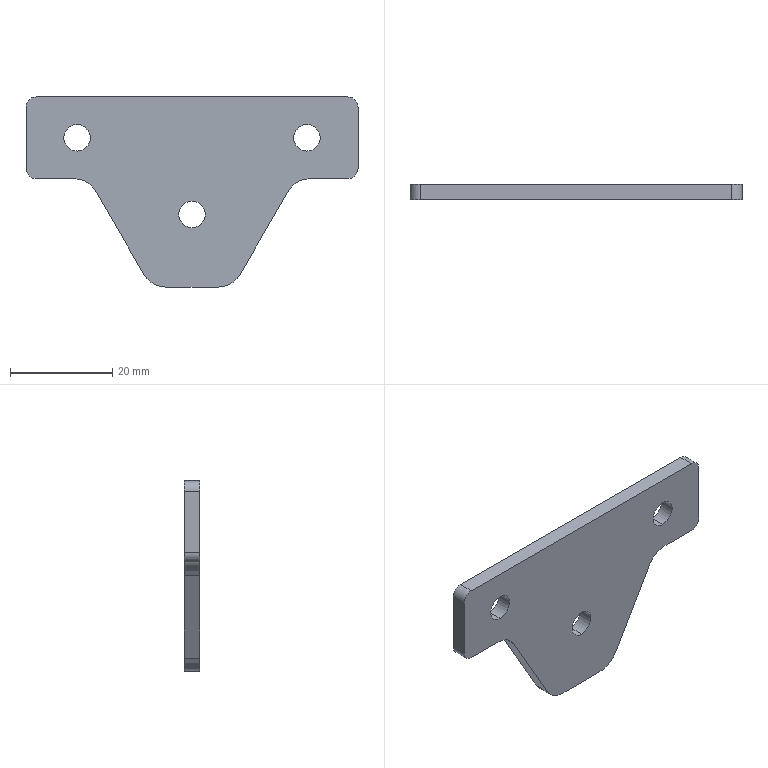Part | SolidWorks | features BaseBody 1 | 1 solid | 24 faces | box 65 x 3 x 37.218 mm | volume 4717 mm3 | cylinder 14 | plane 10 | commonest cylinder face diameters 5.2 x6 4 x4 10 x4
STEP:
#1=CARTESIAN_POINT('',(0.,0.,-17.6));
#2=VERTEX_POINT('',#1);
#3=CARTESIAN_POINT('',(0.,0.,-12.4));
#4=VERTEX_POINT('',#3);
#5=CARTESIAN_POINT('',(0.,0.,-15.));
#6=DIRECTION('',(0.,1.,0.));
#7=DIRECTION('',(0.,0.,1.));
#8=AXIS2_PLACEMENT_3D('',#5,#6,#7);
#9=CIRCLE('',#8,2.6);
#10=EDGE_CURVE('',#2,#4,#9,.T.);
#11=ORIENTED_EDGE('',*,*,#10,.F.);
#12=CARTESIAN_POINT('',(0.,3.,-17.6));
#13=VERTEX_POINT('',#12);
#14=CARTESIAN_POINT('',(0.,0.,-17.6));
#15=DIRECTION('',(0.,1.,0.));
#16=VECTOR('',#15,1000.);
#17=LINE('',#14,#16);
#18=EDGE_CURVE('',#2,#13,#17,.T.);
#19=ORIENTED_EDGE('',*,*,#18,.T.);
#20=CARTESIAN_POINT('',(0.,3.,-12.4));
#21=VERTEX_POINT('',#20);
#22=CARTESIAN_POINT('',(0.,3.,-15.));
#23=DIRECTION('',(0.,-1.,0.));
#24=DIRECTION('',(0.,0.,1.));
#25=AXIS2_PLACEMENT_3D('',#22,#23,#24);
#26=CIRCLE('',#25,2.6);
#27=EDGE_CURVE('',#21,#13,#26,.T.);
#28=ORIENTED_EDGE('',*,*,#27,.F.);
#29=CARTESIAN_POINT('',(0.,0.,-12.4));
#30=DIRECTION('',(0.,1.,0.));
#31=VECTOR('',#30,1000.);
#32=LINE('',#29,#31);
#33=EDGE_CURVE('',#4,#21,#32,.T.);
#34=ORIENTED_EDGE('',*,*,#33,.F.);
#35=EDGE_LOOP('',(#11,#19,#28,#34));
#36=FACE_OUTER_BOUND('',#35,.T.);
#37=CARTESIAN_POINT('',(0.,0.,-15.));
#38=DIRECTION('',(0.,1.,0.));
#39=DIRECTION('',(0.,0.,1.));
#40=AXIS2_PLACEMENT_3D('',#37,#38,#39);
#41=CYLINDRICAL_SURFACE('',#40,2.6);
#42=ADVANCED_FACE('',(#36),#41,.F.);
#43=CARTESIAN_POINT('',(22.5,0.,-2.6));
#44=VERTEX_POINT('',#43);
#45=CARTESIAN_POINT('',(22.5,0.,2.6));
#46=VERTEX_POINT('',#45);
#47=CARTESIAN_POINT('',(22.5,0.,0.));
#48=DIRECTION('',(0.,1.,0.));
#49=DIRECTION('',(0.,0.,1.));
#50=AXIS2_PLACEMENT_3D('',#47,#48,#49);
#51=CIRCLE('',#50,2.6);
#52=EDGE_CURVE('',#44,#46,#51,.T.);
#53=ORIENTED_EDGE('',*,*,#52,.F.);
#54=CARTESIAN_POINT('',(22.5,3.,-2.6));
#55=VERTEX_POINT('',#54);
#56=CARTESIAN_POINT('',(22.5,0.,-2.6));
#57=DIRECTION('',(0.,1.,0.));
#58=VECTOR('',#57,1000.);
#59=LINE('',#56,#58);
#60=EDGE_CURVE('',#44,#55,#59,.T.);
#61=ORIENTED_EDGE('',*,*,#60,.T.);
#62=CARTESIAN_POINT('',(22.5,3.,2.6));
#63=VERTEX_POINT('',#62);
#64=CARTESIAN_POINT('',(22.5,3.,0.));
#65=DIRECTION('',(0.,-1.,0.));
#66=DIRECTION('',(0.,0.,1.));
#67=AXIS2_PLACEMENT_3D('',#64,#65,#66);
#68=CIRCLE('',#67,2.6);
#69=EDGE_CURVE('',#63,#55,#68,.T.);
#70=ORIENTED_EDGE('',*,*,#69,.F.);
#71=CARTESIAN_POINT('',(22.5,0.,2.6));
#72=DIRECTION('',(0.,1.,0.));
#73=VECTOR('',#72,1000.);
#74=LINE('',#71,#73);
#75=EDGE_CURVE('',#46,#63,#74,.T.);
#76=ORIENTED_EDGE('',*,*,#75,.F.);
#77=EDGE_LOOP('',(#53,#61,#70,#76));
#78=FACE_OUTER_BOUND('',#77,.T.);
#79=CARTESIAN_POINT('',(22.5,0.,0.));
#80=DIRECTION('',(0.,1.,0.));
#81=DIRECTION('',(0.,0.,1.));
#82=AXIS2_PLACEMENT_3D('',#79,#80,#81);
#83=CYLINDRICAL_SURFACE('',#82,2.6);
#84=ADVANCED_FACE('',(#78),#83,.F.);
#85=CARTESIAN_POINT('',(-22.5,0.,-2.6));
#86=VERTEX_POINT('',#85);
#87=CARTESIAN_POINT('',(-22.5,0.,2.6));
#88=VERTEX_POINT('',#87);
#89=CARTESIAN_POINT('',(-22.5,0.,0.));
#90=DIRECTION('',(0.,1.,0.));
#91=DIRECTION('',(0.,0.,1.));
#92=AXIS2_PLACEMENT_3D('',#89,#90,#91);
#93=CIRCLE('',#92,2.6);
#94=EDGE_CURVE('',#86,#88,#93,.T.);
#95=ORIENTED_EDGE('',*,*,#94,.F.);
#96=CARTESIAN_POINT('',(-22.5,3.,-2.6));
#97=VERTEX_POINT('',#96);
#98=CARTESIAN_POINT('',(-22.5,0.,-2.6));
#99=DIRECTION('',(0.,1.,0.));
#100=VECTOR('',#99,1000.);
#101=LINE('',#98,#100);
#102=EDGE_CURVE('',#86,#97,#101,.T.);
#103=ORIENTED_EDGE('',*,*,#102,.T.);
#104=CARTESIAN_POINT('',(-22.5,3.,2.6));
#105=VERTEX_POINT('',#104);
#106=CARTESIAN_POINT('',(-22.5,3.,0.));
#107=DIRECTION('',(0.,-1.,0.));
#108=DIRECTION('',(0.,0.,1.));
#109=AXIS2_PLACEMENT_3D('',#106,#107,#108);
#110=CIRCLE('',#109,2.6);
#111=EDGE_CURVE('',#105,#97,#110,.T.);
#112=ORIENTED_EDGE('',*,*,#111,.F.);
#113=CARTESIAN_POINT('',(-22.5,0.,2.6));
#114=DIRECTION('',(0.,1.,0.));
#115=VECTOR('',#114,1000.);
#116=LINE('',#113,#115);
#117=EDGE_CURVE('',#88,#105,#116,.T.);
#118=ORIENTED_EDGE('',*,*,#117,.F.);
#119=EDGE_LOOP('',(#95,#103,#112,#118));
#120=FACE_OUTER_BOUND('',#119,.T.);
#121=CARTESIAN_POINT('',(-22.5,0.,0.));
#122=DIRECTION('',(0.,1.,0.));
#123=DIRECTION('',(0.,0.,1.));
#124=AXIS2_PLACEMENT_3D('',#121,#122,#123);
#125=CYLINDRICAL_SURFACE('',#124,2.6);
#126=ADVANCED_FACE('',(#120),#125,.F.);
#127=ORIENTED_EDGE('',*,*,#27,.T.);
#128=CARTESIAN_POINT('',(0.,3.,-15.));
#129=DIRECTION('',(0.,-1.,0.));
#130=DIRECTION('',(0.,0.,1.));
#131=AXIS2_PLACEMENT_3D('',#128,#129,#130);
#132=CIRCLE('',#131,2.6);
#133=EDGE_CURVE('',#13,#21,#132,.T.);
#134=ORIENTED_EDGE('',*,*,#133,.T.);
#135=EDGE_LOOP('',(#127,#134));
#136=FACE_BOUND('',#135,.T.);
#137=ORIENTED_EDGE('',*,*,#69,.T.);
#138=CARTESIAN_POINT('',(22.5,3.,0.));
#139=DIRECTION('',(0.,-1.,0.));
#140=DIRECTION('',(0.,0.,1.));
#141=AXIS2_PLACEMENT_3D('',#138,#139,#140);
#142=CIRCLE('',#141,2.6);
#143=EDGE_CURVE('',#55,#63,#142,.T.);
#144=ORIENTED_EDGE('',*,*,#143,.T.);
#145=EDGE_LOOP('',(#137,#144));
#146=FACE_BOUND('',#145,.T.);
#147=ORIENTED_EDGE('',*,*,#111,.T.);
#148=CARTESIAN_POINT('',(-22.5,3.,0.));
#149=DIRECTION('',(0.,-1.,0.));
#150=DIRECTION('',(0.,0.,1.));
#151=AXIS2_PLACEMENT_3D('',#148,#149,#150);
#152=CIRCLE('',#151,2.6);
#153=EDGE_CURVE('',#97,#105,#152,.T.);
#154=ORIENTED_EDGE('',*,*,#153,.T.);
#155=EDGE_LOOP('',(#147,#154));
#156=FACE_BOUND('',#155,.T.);
#157=CARTESIAN_POINT('',(30.5,3.,-8.));
#158=VERTEX_POINT('',#157);
#159=CARTESIAN_POINT('',(23.137,3.,-8.));
#160=VERTEX_POINT('',#159);
#161=CARTESIAN_POINT('',(0.,3.,-8.));
#162=DIRECTION('',(-1.,0.,0.));
#163=VECTOR('',#162,1000.);
#164=LINE('',#161,#163);
#165=EDGE_CURVE('',#158,#160,#164,.T.);
#166=ORIENTED_EDGE('',*,*,#165,.T.);
#167=CARTESIAN_POINT('',(18.807,3.,-10.5));
#168=VERTEX_POINT('',#167);
#169=CARTESIAN_POINT('',(23.137,3.,-13.));
#170=DIRECTION('',(0.,-1.,0.));
#171=DIRECTION('',(0.,0.,-1.));
#172=AXIS2_PLACEMENT_3D('',#169,#170,#171);
#173=CIRCLE('',#172,5.);
#174=EDGE_CURVE('',#160,#168,#173,.T.);
#175=ORIENTED_EDGE('',*,*,#174,.T.);
#176=CARTESIAN_POINT('',(9.443,3.,-26.718));
#177=VERTEX_POINT('',#176);
#178=CARTESIAN_POINT('',(18.807,3.,-10.5));
#179=DIRECTION('',(-0.5,0.,-0.866));
#180=VECTOR('',#179,1000.);
#181=LINE('',#178,#180);
#182=EDGE_CURVE('',#168,#177,#181,.T.);
#183=ORIENTED_EDGE('',*,*,#182,.T.);
#184=CARTESIAN_POINT('',(5.113,3.,-29.218));
#185=VERTEX_POINT('',#184);
#186=CARTESIAN_POINT('',(5.113,3.,-24.218));
#187=DIRECTION('',(0.,1.,0.));
#188=DIRECTION('',(0.,0.,-1.));
#189=AXIS2_PLACEMENT_3D('',#186,#187,#188);
#190=CIRCLE('',#189,5.);
#191=EDGE_CURVE('',#177,#185,#190,.T.);
#192=ORIENTED_EDGE('',*,*,#191,.T.);
#193=CARTESIAN_POINT('',(-5.113,3.,-29.218));
#194=VERTEX_POINT('',#193);
#195=CARTESIAN_POINT('',(0.,3.,-29.218));
#196=DIRECTION('',(-1.,0.,0.));
#197=VECTOR('',#196,1000.);
#198=LINE('',#195,#197);
#199=EDGE_CURVE('',#185,#194,#198,.T.);
#200=ORIENTED_EDGE('',*,*,#199,.T.);
#201=CARTESIAN_POINT('',(-9.443,3.,-26.718));
#202=VERTEX_POINT('',#201);
#203=CARTESIAN_POINT('',(-5.113,3.,-24.218));
#204=DIRECTION('',(0.,1.,0.));
#205=DIRECTION('',(0.,0.,1.));
#206=AXIS2_PLACEMENT_3D('',#203,#204,#205);
#207=CIRCLE('',#206,5.);
#208=EDGE_CURVE('',#194,#202,#207,.T.);
#209=ORIENTED_EDGE('',*,*,#208,.T.);
#210=CARTESIAN_POINT('',(-18.807,3.,-10.5));
#211=VERTEX_POINT('',#210);
#212=CARTESIAN_POINT('',(-9.443,3.,-26.718));
#213=DIRECTION('',(-0.5,0.,0.866));
#214=VECTOR('',#213,1000.);
#215=LINE('',#212,#214);
#216=EDGE_CURVE('',#202,#211,#215,.T.);
#217=ORIENTED_EDGE('',*,*,#216,.T.);
#218=CARTESIAN_POINT('',(-23.137,3.,-8.));
#219=VERTEX_POINT('',#218);
#220=CARTESIAN_POINT('',(-23.137,3.,-13.));
#221=DIRECTION('',(0.,-1.,0.));
#222=DIRECTION('',(0.,0.,1.));
#223=AXIS2_PLACEMENT_3D('',#220,#221,#222);
#224=CIRCLE('',#223,5.);
#225=EDGE_CURVE('',#211,#219,#224,.T.);
#226=ORIENTED_EDGE('',*,*,#225,.T.);
#227=CARTESIAN_POINT('',(-30.5,3.,-8.));
#228=VERTEX_POINT('',#227);
#229=CARTESIAN_POINT('',(0.,3.,-8.));
#230=DIRECTION('',(-1.,0.,0.));
#231=VECTOR('',#230,1000.);
#232=LINE('',#229,#231);
#233=EDGE_CURVE('',#219,#228,#232,.T.);
#234=ORIENTED_EDGE('',*,*,#233,.T.);
#235=CARTESIAN_POINT('',(-32.5,3.,-6.));
#236=VERTEX_POINT('',#235);
#237=CARTESIAN_POINT('',(-30.5,3.,-6.));
#238=DIRECTION('',(0.,1.,0.));
#239=DIRECTION('',(0.,0.,-1.));
#240=AXIS2_PLACEMENT_3D('',#237,#238,#239);
#241=CIRCLE('',#240,2.);
#242=EDGE_CURVE('',#228,#236,#241,.T.);
#243=ORIENTED_EDGE('',*,*,#242,.T.);
#244=CARTESIAN_POINT('',(-32.5,3.,6.));
#245=VERTEX_POINT('',#244);
#246=CARTESIAN_POINT('',(-32.5,3.,0.));
#247=DIRECTION('',(0.,0.,1.));
#248=VECTOR('',#247,1000.);
#249=LINE('',#246,#248);
#250=EDGE_CURVE('',#236,#245,#249,.T.);
#251=ORIENTED_EDGE('',*,*,#250,.T.);
#252=CARTESIAN_POINT('',(-30.5,3.,8.));
#253=VERTEX_POINT('',#252);
#254=CARTESIAN_POINT('',(-30.5,3.,6.));
#255=DIRECTION('',(0.,1.,0.));
#256=DIRECTION('',(0.,0.,1.));
#257=AXIS2_PLACEMENT_3D('',#254,#255,#256);
#258=CIRCLE('',#257,2.);
#259=EDGE_CURVE('',#245,#253,#258,.T.);
#260=ORIENTED_EDGE('',*,*,#259,.T.);
#261=CARTESIAN_POINT('',(30.5,3.,8.));
#262=VERTEX_POINT('',#261);
#263=CARTESIAN_POINT('',(0.,3.,8.));
#264=DIRECTION('',(1.,0.,0.));
#265=VECTOR('',#264,1000.);
#266=LINE('',#263,#265);
#267=EDGE_CURVE('',#253,#262,#266,.T.);
#268=ORIENTED_EDGE('',*,*,#267,.T.);
#269=CARTESIAN_POINT('',(32.5,3.,6.));
#270=VERTEX_POINT('',#269);
#271=CARTESIAN_POINT('',(30.5,3.,6.));
#272=DIRECTION('',(0.,1.,0.));
#273=DIRECTION('',(0.,0.,-1.));
#274=AXIS2_PLACEMENT_3D('',#271,#272,#273);
#275=CIRCLE('',#274,2.);
#276=EDGE_CURVE('',#262,#270,#275,.T.);
#277=ORIENTED_EDGE('',*,*,#276,.T.);
#278=CARTESIAN_POINT('',(32.5,3.,-6.));
#279=VERTEX_POINT('',#278);
#280=CARTESIAN_POINT('',(32.5,3.,0.));
#281=DIRECTION('',(0.,0.,-1.));
#282=VECTOR('',#281,1000.);
#283=LINE('',#280,#282);
#284=EDGE_CURVE('',#270,#279,#283,.T.);
#285=ORIENTED_EDGE('',*,*,#284,.T.);
#286=CARTESIAN_POINT('',(30.5,3.,-6.));
#287=DIRECTION('',(0.,1.,0.));
#288=DIRECTION('',(0.,0.,1.));
#289=AXIS2_PLACEMENT_3D('',#286,#287,#288);
#290=CIRCLE('',#289,2.);
#291=EDGE_CURVE('',#279,#158,#290,.T.);
#292=ORIENTED_EDGE('',*,*,#291,.T.);
#293=EDGE_LOOP('',(#166,#175,#183,#192,#200,#209,#217,#226,#234,#243,#251,#260,#268,#277,#285,#292));
#294=FACE_OUTER_BOUND('',#293,.T.);
#295=CARTESIAN_POINT('',(0.,3.,0.));
#296=DIRECTION('',(0.,1.,0.));
#297=DIRECTION('',(0.,0.,1.));
#298=AXIS2_PLACEMENT_3D('',#295,#296,#297);
#299=PLANE('',#298);
#300=ADVANCED_FACE('',(#136,#146,#156,#294),#299,.T.);
#301=ORIENTED_EDGE('',*,*,#18,.F.);
#302=CARTESIAN_POINT('',(0.,0.,-15.));
#303=DIRECTION('',(0.,1.,0.));
#304=DIRECTION('',(0.,0.,1.));
#305=AXIS2_PLACEMENT_3D('',#302,#303,#304);
#306=CIRCLE('',#305,2.6);
#307=EDGE_CURVE('',#4,#2,#306,.T.);
#308=ORIENTED_EDGE('',*,*,#307,.F.);
#309=ORIENTED_EDGE('',*,*,#33,.T.);
#310=ORIENTED_EDGE('',*,*,#133,.F.);
#311=EDGE_LOOP('',(#301,#308,#309,#310));
#312=FACE_OUTER_BOUND('',#311,.T.);
#313=CARTESIAN_POINT('',(0.,0.,-15.));
#314=DIRECTION('',(0.,1.,0.));
#315=DIRECTION('',(0.,0.,1.));
#316=AXIS2_PLACEMENT_3D('',#313,#314,#315);
#317=CYLINDRICAL_SURFACE('',#316,2.6);
#318=ADVANCED_FACE('',(#312),#317,.F.);
#319=ORIENTED_EDGE('',*,*,#60,.F.);
#320=CARTESIAN_POINT('',(22.5,0.,0.));
#321=DIRECTION('',(0.,1.,0.));
#322=DIRECTION('',(0.,0.,1.));
#323=AXIS2_PLACEMENT_3D('',#320,#321,#322);
#324=CIRCLE('',#323,2.6);
#325=EDGE_CURVE('',#46,#44,#324,.T.);
#326=ORIENTED_EDGE('',*,*,#325,.F.);
#327=ORIENTED_EDGE('',*,*,#75,.T.);
#328=ORIENTED_EDGE('',*,*,#143,.F.);
#329=EDGE_LOOP('',(#319,#326,#327,#328));
#330=FACE_OUTER_BOUND('',#329,.T.);
#331=CARTESIAN_POINT('',(22.5,0.,0.));
#332=DIRECTION('',(0.,1.,0.));
#333=DIRECTION('',(0.,0.,1.));
#334=AXIS2_PLACEMENT_3D('',#331,#332,#333);
#335=CYLINDRICAL_SURFACE('',#334,2.6);
#336=ADVANCED_FACE('',(#330),#335,.F.);
#337=ORIENTED_EDGE('',*,*,#102,.F.);
#338=CARTESIAN_POINT('',(-22.5,0.,0.));
#339=DIRECTION('',(0.,1.,0.));
#340=DIRECTION('',(0.,0.,1.));
#341=AXIS2_PLACEMENT_3D('',#338,#339,#340);
#342=CIRCLE('',#341,2.6);
#343=EDGE_CURVE('',#88,#86,#342,.T.);
#344=ORIENTED_EDGE('',*,*,#343,.F.);
#345=ORIENTED_EDGE('',*,*,#117,.T.);
#346=ORIENTED_EDGE('',*,*,#153,.F.);
#347=EDGE_LOOP('',(#337,#344,#345,#346));
#348=FACE_OUTER_BOUND('',#347,.T.);
#349=CARTESIAN_POINT('',(-22.5,0.,0.));
#350=DIRECTION('',(0.,1.,0.));
#351=DIRECTION('',(0.,0.,1.));
#352=AXIS2_PLACEMENT_3D('',#349,#350,#351);
#353=CYLINDRICAL_SURFACE('',#352,2.6);
#354=ADVANCED_FACE('',(#348),#353,.F.);
#355=CARTESIAN_POINT('',(18.807,0.,-10.5));
#356=VERTEX_POINT('',#355);
#357=CARTESIAN_POINT('',(18.807,3.,-10.5));
#358=DIRECTION('',(0.,-1.,0.));
#359=VECTOR('',#358,1000.);
#360=LINE('',#357,#359);
#361=EDGE_CURVE('',#168,#356,#360,.T.);
#362=ORIENTED_EDGE('',*,*,#361,.F.);
#363=ORIENTED_EDGE('',*,*,#174,.F.);
#364=CARTESIAN_POINT('',(23.137,0.,-8.));
#365=VERTEX_POINT('',#364);
#366=CARTESIAN_POINT('',(23.137,3.,-8.));
#367=DIRECTION('',(0.,1.,0.));
#368=VECTOR('',#367,1000.);
#369=LINE('',#366,#368);
#370=EDGE_CURVE('',#365,#160,#369,.T.);
#371=ORIENTED_EDGE('',*,*,#370,.F.);
#372=CARTESIAN_POINT('',(23.137,0.,-13.));
#373=DIRECTION('',(0.,1.,0.));
#374=DIRECTION('',(0.,0.,-1.));
#375=AXIS2_PLACEMENT_3D('',#372,#373,#374);
#376=CIRCLE('',#375,5.);
#377=EDGE_CURVE('',#356,#365,#376,.T.);
#378=ORIENTED_EDGE('',*,*,#377,.F.);
#379=EDGE_LOOP('',(#362,#363,#371,#378));
#380=FACE_OUTER_BOUND('',#379,.T.);
#381=CARTESIAN_POINT('',(23.137,3.,-13.));
#382=DIRECTION('',(0.,-1.,0.));
#383=DIRECTION('',(0.,0.,-1.));
#384=AXIS2_PLACEMENT_3D('',#381,#382,#383);
#385=CYLINDRICAL_SURFACE('',#384,5.);
#386=ADVANCED_FACE('',(#380),#385,.F.);
#387=ORIENTED_EDGE('',*,*,#165,.F.);
#388=CARTESIAN_POINT('',(30.5,0.,-8.));
#389=VERTEX_POINT('',#388);
#390=CARTESIAN_POINT('',(30.5,3.,-8.));
#391=DIRECTION('',(0.,-1.,0.));
#392=VECTOR('',#391,1000.);
#393=LINE('',#390,#392);
#394=EDGE_CURVE('',#158,#389,#393,.T.);
#395=ORIENTED_EDGE('',*,*,#394,.T.);
#396=CARTESIAN_POINT('',(-32.5,0.,-8.));
#397=DIRECTION('',(-1.,0.,0.));
#398=VECTOR('',#397,1000.);
#399=LINE('',#396,#398);
#400=EDGE_CURVE('',#389,#365,#399,.T.);
#401=ORIENTED_EDGE('',*,*,#400,.T.);
#402=ORIENTED_EDGE('',*,*,#370,.T.);
#403=EDGE_LOOP('',(#387,#395,#401,#402));
#404=FACE_OUTER_BOUND('',#403,.T.);
#405=CARTESIAN_POINT('',(-32.5,3.,-8.));
#406=DIRECTION('',(0.,0.,-1.));
#407=DIRECTION('',(-1.,0.,0.));
#408=AXIS2_PLACEMENT_3D('',#405,#406,#407);
#409=PLANE('',#408);
#410=ADVANCED_FACE('',(#404),#409,.T.);
#411=CARTESIAN_POINT('',(32.5,0.,-6.));
#412=VERTEX_POINT('',#411);
#413=CARTESIAN_POINT('',(30.5,0.,-6.));
#414=DIRECTION('',(0.,1.,0.));
#415=DIRECTION('',(0.,0.,1.));
#416=AXIS2_PLACEMENT_3D('',#413,#414,#415);
#417=CIRCLE('',#416,2.);
#418=EDGE_CURVE('',#412,#389,#417,.T.);
#419=ORIENTED_EDGE('',*,*,#418,.T.);
#420=ORIENTED_EDGE('',*,*,#394,.F.);
#421=ORIENTED_EDGE('',*,*,#291,.F.);
#422=CARTESIAN_POINT('',(32.5,3.,-6.));
#423=DIRECTION('',(0.,-1.,0.));
#424=VECTOR('',#423,1000.);
#425=LINE('',#422,#424);
#426=EDGE_CURVE('',#279,#412,#425,.T.);
#427=ORIENTED_EDGE('',*,*,#426,.T.);
#428=EDGE_LOOP('',(#419,#420,#421,#427));
#429=FACE_OUTER_BOUND('',#428,.T.);
#430=CARTESIAN_POINT('',(30.5,3.,-6.));
#431=DIRECTION('',(0.,1.,0.));
#432=DIRECTION('',(0.,0.,1.));
#433=AXIS2_PLACEMENT_3D('',#430,#431,#432);
#434=CYLINDRICAL_SURFACE('',#433,2.);
#435=ADVANCED_FACE('',(#429),#434,.T.);
#436=ORIENTED_EDGE('',*,*,#426,.F.);
#437=ORIENTED_EDGE('',*,*,#284,.F.);
#438=CARTESIAN_POINT('',(32.5,0.,6.));
#439=VERTEX_POINT('',#438);
#440=CARTESIAN_POINT('',(32.5,3.,6.));
#441=DIRECTION('',(0.,1.,0.));
#442=VECTOR('',#441,1000.);
#443=LINE('',#440,#442);
#444=EDGE_CURVE('',#439,#270,#443,.T.);
#445=ORIENTED_EDGE('',*,*,#444,.F.);
#446=CARTESIAN_POINT('',(32.5,0.,8.));
#447=DIRECTION('',(0.,0.,1.));
#448=VECTOR('',#447,1000.);
#449=LINE('',#446,#448);
#450=EDGE_CURVE('',#412,#439,#449,.T.);
#451=ORIENTED_EDGE('',*,*,#450,.F.);
#452=EDGE_LOOP('',(#436,#437,#445,#451));
#453=FACE_OUTER_BOUND('',#452,.T.);
#454=CARTESIAN_POINT('',(32.5,3.,8.));
#455=DIRECTION('',(-1.,0.,0.));
#456=DIRECTION('',(0.,0.,1.));
#457=AXIS2_PLACEMENT_3D('',#454,#455,#456);
#458=PLANE('',#457);
#459=ADVANCED_FACE('',(#453),#458,.F.);
#460=CARTESIAN_POINT('',(30.5,0.,8.));
#461=VERTEX_POINT('',#460);
#462=CARTESIAN_POINT('',(30.5,0.,6.));
#463=DIRECTION('',(0.,1.,0.));
#464=DIRECTION('',(0.,0.,-1.));
#465=AXIS2_PLACEMENT_3D('',#462,#463,#464);
#466=CIRCLE('',#465,2.);
#467=EDGE_CURVE('',#461,#439,#466,.T.);
#468=ORIENTED_EDGE('',*,*,#467,.T.);
#469=ORIENTED_EDGE('',*,*,#444,.T.);
#470=ORIENTED_EDGE('',*,*,#276,.F.);
#471=CARTESIAN_POINT('',(30.5,3.,8.));
#472=DIRECTION('',(0.,-1.,0.));
#473=VECTOR('',#472,1000.);
#474=LINE('',#471,#473);
#475=EDGE_CURVE('',#262,#461,#474,.T.);
#476=ORIENTED_EDGE('',*,*,#475,.T.);
#477=EDGE_LOOP('',(#468,#469,#470,#476));
#478=FACE_OUTER_BOUND('',#477,.T.);
#479=CARTESIAN_POINT('',(30.5,3.,6.));
#480=DIRECTION('',(0.,-1.,0.));
#481=DIRECTION('',(0.,0.,-1.));
#482=AXIS2_PLACEMENT_3D('',#479,#480,#481);
#483=CYLINDRICAL_SURFACE('',#482,2.);
#484=ADVANCED_FACE('',(#478),#483,.T.);
#485=ORIENTED_EDGE('',*,*,#475,.F.);
#486=ORIENTED_EDGE('',*,*,#267,.F.);
#487=CARTESIAN_POINT('',(-30.5,0.,8.));
#488=VERTEX_POINT('',#487);
#489=CARTESIAN_POINT('',(-30.5,3.,8.));
#490=DIRECTION('',(0.,1.,0.));
#491=VECTOR('',#490,1000.);
#492=LINE('',#489,#491);
#493=EDGE_CURVE('',#488,#253,#492,.T.);
#494=ORIENTED_EDGE('',*,*,#493,.F.);
#495=CARTESIAN_POINT('',(-32.5,0.,8.));
#496=DIRECTION('',(-1.,0.,0.));
#497=VECTOR('',#496,1000.);
#498=LINE('',#495,#497);
#499=EDGE_CURVE('',#461,#488,#498,.T.);
#500=ORIENTED_EDGE('',*,*,#499,.F.);
#501=EDGE_LOOP('',(#485,#486,#494,#500));
#502=FACE_OUTER_BOUND('',#501,.T.);
#503=CARTESIAN_POINT('',(-32.5,3.,8.));
#504=DIRECTION('',(0.,0.,-1.));
#505=DIRECTION('',(-1.,0.,0.));
#506=AXIS2_PLACEMENT_3D('',#503,#504,#505);
#507=PLANE('',#506);
#508=ADVANCED_FACE('',(#502),#507,.F.);
#509=CARTESIAN_POINT('',(-32.5,0.,6.));
#510=VERTEX_POINT('',#509);
#511=CARTESIAN_POINT('',(-30.5,0.,6.));
#512=DIRECTION('',(0.,1.,0.));
#513=DIRECTION('',(0.,0.,1.));
#514=AXIS2_PLACEMENT_3D('',#511,#512,#513);
#515=CIRCLE('',#514,2.);
#516=EDGE_CURVE('',#510,#488,#515,.T.);
#517=ORIENTED_EDGE('',*,*,#516,.T.);
#518=ORIENTED_EDGE('',*,*,#493,.T.);
#519=ORIENTED_EDGE('',*,*,#259,.F.);
#520=CARTESIAN_POINT('',(-32.5,3.,6.));
#521=DIRECTION('',(0.,-1.,0.));
#522=VECTOR('',#521,1000.);
#523=LINE('',#520,#522);
#524=EDGE_CURVE('',#245,#510,#523,.T.);
#525=ORIENTED_EDGE('',*,*,#524,.T.);
#526=EDGE_LOOP('',(#517,#518,#519,#525));
#527=FACE_OUTER_BOUND('',#526,.T.);
#528=CARTESIAN_POINT('',(-30.5,3.,6.));
#529=DIRECTION('',(0.,1.,0.));
#530=DIRECTION('',(0.,0.,1.));
#531=AXIS2_PLACEMENT_3D('',#528,#529,#530);
#532=CYLINDRICAL_SURFACE('',#531,2.);
#533=ADVANCED_FACE('',(#527),#532,.T.);
#534=ORIENTED_EDGE('',*,*,#250,.F.);
#535=CARTESIAN_POINT('',(-32.5,0.,-6.));
#536=VERTEX_POINT('',#535);
#537=CARTESIAN_POINT('',(-32.5,3.,-6.));
#538=DIRECTION('',(0.,-1.,0.));
#539=VECTOR('',#538,1000.);
#540=LINE('',#537,#539);
#541=EDGE_CURVE('',#236,#536,#540,.T.);
#542=ORIENTED_EDGE('',*,*,#541,.T.);
#543=CARTESIAN_POINT('',(-32.5,0.,8.));
#544=DIRECTION('',(0.,0.,1.));
#545=VECTOR('',#544,1000.);
#546=LINE('',#543,#545);
#547=EDGE_CURVE('',#536,#510,#546,.T.);
#548=ORIENTED_EDGE('',*,*,#547,.T.);
#549=ORIENTED_EDGE('',*,*,#524,.F.);
#550=EDGE_LOOP('',(#534,#542,#548,#549));
#551=FACE_OUTER_BOUND('',#550,.T.);
#552=CARTESIAN_POINT('',(-32.5,3.,8.));
#553=DIRECTION('',(-1.,0.,0.));
#554=DIRECTION('',(0.,0.,1.));
#555=AXIS2_PLACEMENT_3D('',#552,#553,#554);
#556=PLANE('',#555);
#557=ADVANCED_FACE('',(#551),#556,.T.);
#558=CARTESIAN_POINT('',(-30.5,0.,-8.));
#559=VERTEX_POINT('',#558);
#560=CARTESIAN_POINT('',(-30.5,0.,-6.));
#561=DIRECTION('',(0.,1.,0.));
#562=DIRECTION('',(0.,0.,-1.));
#563=AXIS2_PLACEMENT_3D('',#560,#561,#562);
#564=CIRCLE('',#563,2.);
#565=EDGE_CURVE('',#559,#536,#564,.T.);
#566=ORIENTED_EDGE('',*,*,#565,.T.);
#567=ORIENTED_EDGE('',*,*,#541,.F.);
#568=ORIENTED_EDGE('',*,*,#242,.F.);
#569=CARTESIAN_POINT('',(-30.5,3.,-8.));
#570=DIRECTION('',(0.,-1.,0.));
#571=VECTOR('',#570,1000.);
#572=LINE('',#569,#571);
#573=EDGE_CURVE('',#228,#559,#572,.T.);
#574=ORIENTED_EDGE('',*,*,#573,.T.);
#575=EDGE_LOOP('',(#566,#567,#568,#574));
#576=FACE_OUTER_BOUND('',#575,.T.);
#577=CARTESIAN_POINT('',(-30.5,3.,-6.));
#578=DIRECTION('',(0.,-1.,0.));
#579=DIRECTION('',(0.,0.,-1.));
#580=AXIS2_PLACEMENT_3D('',#577,#578,#579);
#581=CYLINDRICAL_SURFACE('',#580,2.);
#582=ADVANCED_FACE('',(#576),#581,.T.);
#583=CARTESIAN_POINT('',(-23.137,0.,-8.));
#584=VERTEX_POINT('',#583);
#585=CARTESIAN_POINT('',(-32.5,0.,-8.));
#586=DIRECTION('',(-1.,0.,0.));
#587=VECTOR('',#586,1000.);
#588=LINE('',#585,#587);
#589=EDGE_CURVE('',#584,#559,#588,.T.);
#590=ORIENTED_EDGE('',*,*,#589,.T.);
#591=ORIENTED_EDGE('',*,*,#573,.F.);
#592=ORIENTED_EDGE('',*,*,#233,.F.);
#593=CARTESIAN_POINT('',(-23.137,3.,-8.));
#594=DIRECTION('',(0.,-1.,0.));
#595=VECTOR('',#594,1000.);
#596=LINE('',#593,#595);
#597=EDGE_CURVE('',#219,#584,#596,.T.);
#598=ORIENTED_EDGE('',*,*,#597,.T.);
#599=EDGE_LOOP('',(#590,#591,#592,#598));
#600=FACE_OUTER_BOUND('',#599,.T.);
#601=CARTESIAN_POINT('',(-32.5,3.,-8.));
#602=DIRECTION('',(0.,0.,-1.));
#603=DIRECTION('',(-1.,0.,0.));
#604=AXIS2_PLACEMENT_3D('',#601,#602,#603);
#605=PLANE('',#604);
#606=ADVANCED_FACE('',(#600),#605,.T.);
#607=ORIENTED_EDGE('',*,*,#597,.F.);
#608=ORIENTED_EDGE('',*,*,#225,.F.);
#609=CARTESIAN_POINT('',(-18.807,0.,-10.5));
#610=VERTEX_POINT('',#609);
#611=CARTESIAN_POINT('',(-18.807,-24.5,-10.5));
#612=DIRECTION('',(0.,1.,0.));
#613=VECTOR('',#612,1000.);
#614=LINE('',#611,#613);
#615=EDGE_CURVE('',#610,#211,#614,.T.);
#616=ORIENTED_EDGE('',*,*,#615,.F.);
#617=CARTESIAN_POINT('',(-23.137,0.,-13.));
#618=DIRECTION('',(0.,1.,0.));
#619=DIRECTION('',(0.,0.,1.));
#620=AXIS2_PLACEMENT_3D('',#617,#618,#619);
#621=CIRCLE('',#620,5.);
#622=EDGE_CURVE('',#584,#610,#621,.T.);
#623=ORIENTED_EDGE('',*,*,#622,.F.);
#624=EDGE_LOOP('',(#607,#608,#616,#623));
#625=FACE_OUTER_BOUND('',#624,.T.);
#626=CARTESIAN_POINT('',(-23.137,-24.5,-13.));
#627=DIRECTION('',(0.,1.,0.));
#628=DIRECTION('',(0.,0.,1.));
#629=AXIS2_PLACEMENT_3D('',#626,#627,#628);
#630=CYLINDRICAL_SURFACE('',#629,5.);
#631=ADVANCED_FACE('',(#625),#630,.F.);
#632=CARTESIAN_POINT('',(-9.443,0.,-26.718));
#633=VERTEX_POINT('',#632);
#634=CARTESIAN_POINT('',(-9.443,-24.5,-26.718));
#635=DIRECTION('',(0.,1.,0.));
#636=VECTOR('',#635,1000.);
#637=LINE('',#634,#636);
#638=EDGE_CURVE('',#633,#202,#637,.T.);
#639=ORIENTED_EDGE('',*,*,#638,.F.);
#640=CARTESIAN_POINT('',(-18.652,0.,-10.769));
#641=DIRECTION('',(0.5,0.,-0.866));
#642=VECTOR('',#641,1000.);
#643=LINE('',#640,#642);
#644=EDGE_CURVE('',#610,#633,#643,.T.);
#645=ORIENTED_EDGE('',*,*,#644,.F.);
#646=ORIENTED_EDGE('',*,*,#615,.T.);
#647=ORIENTED_EDGE('',*,*,#216,.F.);
#648=EDGE_LOOP('',(#639,#645,#646,#647));
#649=FACE_OUTER_BOUND('',#648,.T.);
#650=CARTESIAN_POINT('',(-18.652,-24.5,-10.769));
#651=DIRECTION('',(0.866,0.,0.5));
#652=DIRECTION('',(0.5,0.,-0.866));
#653=AXIS2_PLACEMENT_3D('',#650,#651,#652);
#654=PLANE('',#653);
#655=ADVANCED_FACE('',(#649),#654,.F.);
#656=ORIENTED_EDGE('',*,*,#208,.F.);
#657=CARTESIAN_POINT('',(-5.113,0.,-29.218));
#658=VERTEX_POINT('',#657);
#659=CARTESIAN_POINT('',(-5.113,-7.,-29.218));
#660=DIRECTION('',(0.,-1.,0.));
#661=VECTOR('',#660,1000.);
#662=LINE('',#659,#661);
#663=EDGE_CURVE('',#194,#658,#662,.T.);
#664=ORIENTED_EDGE('',*,*,#663,.T.);
#665=CARTESIAN_POINT('',(-5.113,0.,-24.218));
#666=DIRECTION('',(0.,1.,0.));
#667=DIRECTION('',(0.,0.,1.));
#668=AXIS2_PLACEMENT_3D('',#665,#666,#667);
#669=CIRCLE('',#668,5.);
#670=EDGE_CURVE('',#658,#633,#669,.T.);
#671=ORIENTED_EDGE('',*,*,#670,.T.);
#672=ORIENTED_EDGE('',*,*,#638,.T.);
#673=EDGE_LOOP('',(#656,#664,#671,#672));
#674=FACE_OUTER_BOUND('',#673,.T.);
#675=CARTESIAN_POINT('',(-5.113,-7.,-24.218));
#676=DIRECTION('',(0.,1.,0.));
#677=DIRECTION('',(0.,0.,1.));
#678=AXIS2_PLACEMENT_3D('',#675,#676,#677);
#679=CYLINDRICAL_SURFACE('',#678,5.);
#680=ADVANCED_FACE('',(#674),#679,.T.);
#681=CARTESIAN_POINT('',(5.113,0.,-29.218));
#682=VERTEX_POINT('',#681);
#683=CARTESIAN_POINT('',(5.113,-7.,-29.218));
#684=DIRECTION('',(0.,1.,0.));
#685=VECTOR('',#684,1000.);
#686=LINE('',#683,#685);
#687=EDGE_CURVE('',#682,#185,#686,.T.);
#688=ORIENTED_EDGE('',*,*,#687,.F.);
#689=CARTESIAN_POINT('',(-8.,0.,-29.218));
#690=DIRECTION('',(1.,0.,0.));
#691=VECTOR('',#690,1000.);
#692=LINE('',#689,#691);
#693=EDGE_CURVE('',#658,#682,#692,.T.);
#694=ORIENTED_EDGE('',*,*,#693,.F.);
#695=ORIENTED_EDGE('',*,*,#663,.F.);
#696=ORIENTED_EDGE('',*,*,#199,.F.);
#697=EDGE_LOOP('',(#688,#694,#695,#696));
#698=FACE_OUTER_BOUND('',#697,.T.);
#699=CARTESIAN_POINT('',(-8.,-7.,-29.218));
#700=DIRECTION('',(0.,0.,1.));
#701=DIRECTION('',(1.,0.,0.));
#702=AXIS2_PLACEMENT_3D('',#699,#700,#701);
#703=PLANE('',#702);
#704=ADVANCED_FACE('',(#698),#703,.F.);
#705=ORIENTED_EDGE('',*,*,#191,.F.);
#706=CARTESIAN_POINT('',(9.443,0.,-26.718));
#707=VERTEX_POINT('',#706);
#708=CARTESIAN_POINT('',(9.443,-24.5,-26.718));
#709=DIRECTION('',(0.,-1.,0.));
#710=VECTOR('',#709,1000.);
#711=LINE('',#708,#710);
#712=EDGE_CURVE('',#177,#707,#711,.T.);
#713=ORIENTED_EDGE('',*,*,#712,.T.);
#714=CARTESIAN_POINT('',(5.113,0.,-24.218));
#715=DIRECTION('',(0.,1.,0.));
#716=DIRECTION('',(0.,0.,-1.));
#717=AXIS2_PLACEMENT_3D('',#714,#715,#716);
#718=CIRCLE('',#717,5.);
#719=EDGE_CURVE('',#707,#682,#718,.T.);
#720=ORIENTED_EDGE('',*,*,#719,.T.);
#721=ORIENTED_EDGE('',*,*,#687,.T.);
#722=EDGE_LOOP('',(#705,#713,#720,#721));
#723=FACE_OUTER_BOUND('',#722,.T.);
#724=CARTESIAN_POINT('',(5.113,-24.5,-24.218));
#725=DIRECTION('',(0.,-1.,0.));
#726=DIRECTION('',(0.,0.,-1.));
#727=AXIS2_PLACEMENT_3D('',#724,#725,#726);
#728=CYLINDRICAL_SURFACE('',#727,5.);
#729=ADVANCED_FACE('',(#723),#728,.T.);
#730=ORIENTED_EDGE('',*,*,#182,.F.);
#731=ORIENTED_EDGE('',*,*,#361,.T.);
#732=CARTESIAN_POINT('',(18.652,0.,-10.769));
#733=DIRECTION('',(-0.5,0.,-0.866));
#734=VECTOR('',#733,1000.);
#735=LINE('',#732,#734);
#736=EDGE_CURVE('',#356,#707,#735,.T.);
#737=ORIENTED_EDGE('',*,*,#736,.T.);
#738=ORIENTED_EDGE('',*,*,#712,.F.);
#739=EDGE_LOOP('',(#730,#731,#737,#738));
#740=FACE_OUTER_BOUND('',#739,.T.);
#741=CARTESIAN_POINT('',(18.652,-24.5,-10.769));
#742=DIRECTION('',(0.866,0.,-0.5));
#743=DIRECTION('',(-0.5,0.,-0.866));
#744=AXIS2_PLACEMENT_3D('',#741,#742,#743);
#745=PLANE('',#744);
#746=ADVANCED_FACE('',(#740),#745,.T.);
#747=ORIENTED_EDGE('',*,*,#307,.T.);
#748=ORIENTED_EDGE('',*,*,#10,.T.);
#749=EDGE_LOOP('',(#747,#748));
#750=FACE_BOUND('',#749,.T.);
#751=ORIENTED_EDGE('',*,*,#325,.T.);
#752=ORIENTED_EDGE('',*,*,#52,.T.);
#753=EDGE_LOOP('',(#751,#752));
#754=FACE_BOUND('',#753,.T.);
#755=ORIENTED_EDGE('',*,*,#343,.T.);
#756=ORIENTED_EDGE('',*,*,#94,.T.);
#757=EDGE_LOOP('',(#755,#756));
#758=FACE_BOUND('',#757,.T.);
#759=ORIENTED_EDGE('',*,*,#719,.F.);
#760=ORIENTED_EDGE('',*,*,#736,.F.);
#761=ORIENTED_EDGE('',*,*,#377,.T.);
#762=ORIENTED_EDGE('',*,*,#400,.F.);
#763=ORIENTED_EDGE('',*,*,#418,.F.);
#764=ORIENTED_EDGE('',*,*,#450,.T.);
#765=ORIENTED_EDGE('',*,*,#467,.F.);
#766=ORIENTED_EDGE('',*,*,#499,.T.);
#767=ORIENTED_EDGE('',*,*,#516,.F.);
#768=ORIENTED_EDGE('',*,*,#547,.F.);
#769=ORIENTED_EDGE('',*,*,#565,.F.);
#770=ORIENTED_EDGE('',*,*,#589,.F.);
#771=ORIENTED_EDGE('',*,*,#622,.T.);
#772=ORIENTED_EDGE('',*,*,#644,.T.);
#773=ORIENTED_EDGE('',*,*,#670,.F.);
#774=ORIENTED_EDGE('',*,*,#693,.T.);
#775=EDGE_LOOP('',(#759,#760,#761,#762,#763,#764,#765,#766,#767,#768,#769,#770,#771,#772,#773,#774));
#776=FACE_OUTER_BOUND('',#775,.T.);
#777=CARTESIAN_POINT('',(0.,0.,0.));
#778=DIRECTION('',(0.,1.,0.));
#779=DIRECTION('',(0.,0.,1.));
#780=AXIS2_PLACEMENT_3D('',#777,#778,#779);
#781=PLANE('',#780);
#782=ADVANCED_FACE('',(#750,#754,#758,#776),#781,.F.);
#783=CLOSED_SHELL('',(#42,#84,#126,#300,#318,#336,#354,#386,#410,#435,#459,#484,#508,#533,#557,#582,#606,#631,#655,#680,#704,#729,#746,#782));
#784=MANIFOLD_SOLID_BREP('',#783);
#785=CARTESIAN_POINT('',(0.,0.,0.));
#786=DIRECTION('',(0.,0.,1.));
#787=DIRECTION('',(1.,0.,0.));
#788=AXIS2_PLACEMENT_3D('',#785,#786,#787);
#789=(LENGTH_UNIT()NAMED_UNIT(*)SI_UNIT(.MILLI.,.METRE.));
#790=UNCERTAINTY_MEASURE_WITH_UNIT(LENGTH_MEASURE(0.00001),#789,'','');
#791=(NAMED_UNIT(*)PLANE_ANGLE_UNIT()SI_UNIT($,.RADIAN.));
#792=(NAMED_UNIT(*)SI_UNIT($,.STERADIAN.)SOLID_ANGLE_UNIT());
#793=(GEOMETRIC_REPRESENTATION_CONTEXT(3)GLOBAL_UNCERTAINTY_ASSIGNED_CONTEXT((#790))GLOBAL_UNIT_ASSIGNED_CONTEXT((#789,#791,#792))REPRESENTATION_CONTEXT('',''));
#794=ADVANCED_BREP_SHAPE_REPRESENTATION('',(#784,#788),#793);